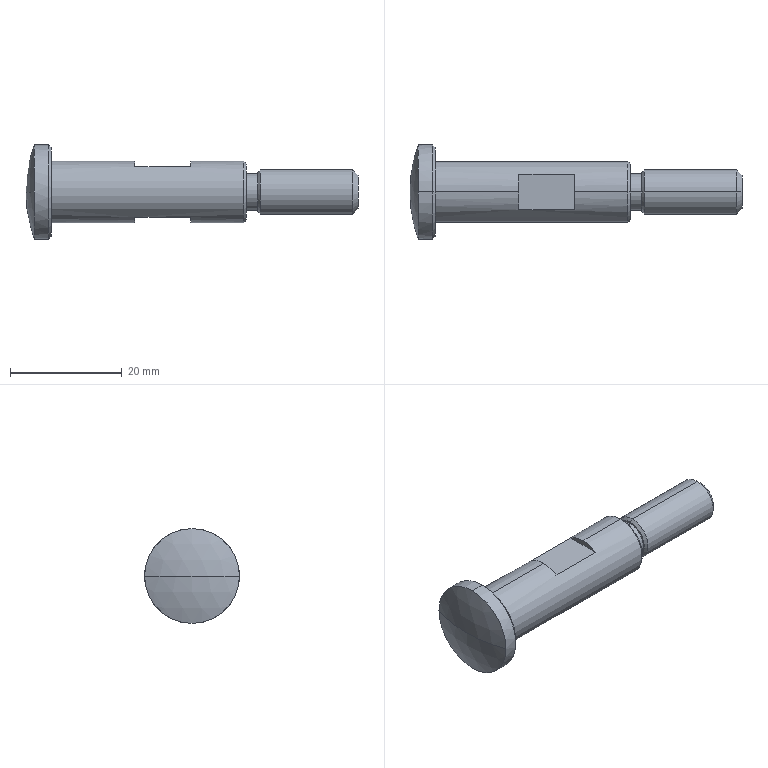Part | SolidWorks | features Chamfer 2, ICE 1, MirrorPattern 1, RefAxis 1, RevCut 1, Revolution 1 | 1 solid | 28 faces | box 59.5 x 17 x 17 mm | volume 5040 mm3 | plane 10 | cone 8 | cylinder 8 | sphere 2 | commonest cylinder face diameters 6.5 x2 8 x2 11 x2 17 x2
STEP:
#1=CARTESIAN_POINT('',(41.5,0.,3.5));
#2=VERTEX_POINT('',#1);
#3=CARTESIAN_POINT('',(41.5,0.,-3.5));
#4=VERTEX_POINT('',#3);
#5=CARTESIAN_POINT('',(41.5,0.,0.));
#6=DIRECTION('',(-1.,0.,0.));
#7=DIRECTION('',(0.,0.,-1.));
#8=AXIS2_PLACEMENT_3D('',#5,#6,#7);
#9=CIRCLE('',#8,3.5);
#10=EDGE_CURVE('',#2,#4,#9,.T.);
#11=ORIENTED_EDGE('',*,*,#10,.F.);
#12=CARTESIAN_POINT('',(42.,0.,4.));
#13=VERTEX_POINT('',#12);
#14=CARTESIAN_POINT('',(42.,0.,4.));
#15=DIRECTION('',(0.7071,0.,0.7071));
#16=VECTOR('',#15,1000.);
#17=LINE('',#14,#16);
#18=EDGE_CURVE('',#2,#13,#17,.T.);
#19=ORIENTED_EDGE('',*,*,#18,.T.);
#20=CARTESIAN_POINT('',(42.,0.,-4.));
#21=VERTEX_POINT('',#20);
#22=CARTESIAN_POINT('',(42.,0.,0.));
#23=DIRECTION('',(1.,0.,0.));
#24=DIRECTION('',(0.,0.,-1.));
#25=AXIS2_PLACEMENT_3D('',#22,#23,#24);
#26=CIRCLE('',#25,4.);
#27=EDGE_CURVE('',#21,#13,#26,.T.);
#28=ORIENTED_EDGE('',*,*,#27,.F.);
#29=CARTESIAN_POINT('',(42.,0.,-4.));
#30=DIRECTION('',(0.7071,0.,-0.7071));
#31=VECTOR('',#30,1000.);
#32=LINE('',#29,#31);
#33=EDGE_CURVE('',#4,#21,#32,.T.);
#34=ORIENTED_EDGE('',*,*,#33,.F.);
#35=EDGE_LOOP('',(#11,#19,#28,#34));
#36=FACE_OUTER_BOUND('',#35,.T.);
#37=CARTESIAN_POINT('',(42.,0.,0.));
#38=DIRECTION('',(1.,0.,0.));
#39=DIRECTION('',(0.,0.,-1.));
#40=AXIS2_PLACEMENT_3D('',#37,#38,#39);
#41=CONICAL_SURFACE('',#40,4.,0.7854);
#42=ADVANCED_FACE('',(#36),#41,.T.);
#43=CARTESIAN_POINT('',(58.5,0.,4.));
#44=VERTEX_POINT('',#43);
#45=CARTESIAN_POINT('',(58.5,0.,-4.));
#46=VERTEX_POINT('',#45);
#47=CARTESIAN_POINT('',(58.5,0.,0.));
#48=DIRECTION('',(-1.,0.,0.));
#49=DIRECTION('',(0.,0.,1.));
#50=AXIS2_PLACEMENT_3D('',#47,#48,#49);
#51=CIRCLE('',#50,4.);
#52=EDGE_CURVE('',#44,#46,#51,.T.);
#53=ORIENTED_EDGE('',*,*,#52,.T.);
#54=CARTESIAN_POINT('',(0.,0.,-4.));
#55=DIRECTION('',(-1.,0.,0.));
#56=VECTOR('',#55,1000.);
#57=LINE('',#54,#56);
#58=EDGE_CURVE('',#46,#21,#57,.T.);
#59=ORIENTED_EDGE('',*,*,#58,.T.);
#60=ORIENTED_EDGE('',*,*,#27,.T.);
#61=CARTESIAN_POINT('',(0.,0.,4.));
#62=DIRECTION('',(-1.,0.,0.));
#63=VECTOR('',#62,1000.);
#64=LINE('',#61,#63);
#65=EDGE_CURVE('',#44,#13,#64,.T.);
#66=ORIENTED_EDGE('',*,*,#65,.F.);
#67=EDGE_LOOP('',(#53,#59,#60,#66));
#68=FACE_OUTER_BOUND('',#67,.T.);
#69=CARTESIAN_POINT('',(0.,0.,0.));
#70=DIRECTION('',(-1.,0.,0.));
#71=DIRECTION('',(0.,0.,1.));
#72=AXIS2_PLACEMENT_3D('',#69,#70,#71);
#73=CYLINDRICAL_SURFACE('',#72,4.);
#74=ADVANCED_FACE('',(#68),#73,.T.);
#75=CARTESIAN_POINT('',(59.5,0.,3.));
#76=VERTEX_POINT('',#75);
#77=CARTESIAN_POINT('',(59.5,0.,-3.));
#78=VERTEX_POINT('',#77);
#79=CARTESIAN_POINT('',(59.5,0.,0.));
#80=DIRECTION('',(-1.,0.,0.));
#81=DIRECTION('',(0.,0.,1.));
#82=AXIS2_PLACEMENT_3D('',#79,#80,#81);
#83=CIRCLE('',#82,3.);
#84=EDGE_CURVE('',#76,#78,#83,.T.);
#85=ORIENTED_EDGE('',*,*,#84,.T.);
#86=CARTESIAN_POINT('',(59.5,0.,-3.));
#87=DIRECTION('',(-0.7071,0.,-0.7071));
#88=VECTOR('',#87,1000.);
#89=LINE('',#86,#88);
#90=EDGE_CURVE('',#78,#46,#89,.T.);
#91=ORIENTED_EDGE('',*,*,#90,.T.);
#92=ORIENTED_EDGE('',*,*,#52,.F.);
#93=CARTESIAN_POINT('',(59.5,0.,3.));
#94=DIRECTION('',(-0.7071,0.,0.7071));
#95=VECTOR('',#94,1000.);
#96=LINE('',#93,#95);
#97=EDGE_CURVE('',#76,#44,#96,.T.);
#98=ORIENTED_EDGE('',*,*,#97,.F.);
#99=EDGE_LOOP('',(#85,#91,#92,#98));
#100=FACE_OUTER_BOUND('',#99,.T.);
#101=CARTESIAN_POINT('',(59.5,0.,0.));
#102=DIRECTION('',(-1.,0.,0.));
#103=DIRECTION('',(0.,0.,1.));
#104=AXIS2_PLACEMENT_3D('',#101,#102,#103);
#105=CONICAL_SURFACE('',#104,3.,0.7854);
#106=ADVANCED_FACE('',(#100),#105,.T.);
#107=CARTESIAN_POINT('',(39.5,0.,-3.25));
#108=VERTEX_POINT('',#107);
#109=CARTESIAN_POINT('',(39.5,0.,3.25));
#110=VERTEX_POINT('',#109);
#111=CARTESIAN_POINT('',(39.5,0.,0.));
#112=DIRECTION('',(1.,0.,0.));
#113=DIRECTION('',(0.,0.,-1.));
#114=AXIS2_PLACEMENT_3D('',#111,#112,#113);
#115=CIRCLE('',#114,3.25);
#116=EDGE_CURVE('',#108,#110,#115,.T.);
#117=ORIENTED_EDGE('',*,*,#116,.T.);
#118=CARTESIAN_POINT('',(41.5,0.,3.25));
#119=VERTEX_POINT('',#118);
#120=CARTESIAN_POINT('',(58.5,0.,3.25));
#121=DIRECTION('',(1.,0.,0.));
#122=VECTOR('',#121,1000.);
#123=LINE('',#120,#122);
#124=EDGE_CURVE('',#110,#119,#123,.T.);
#125=ORIENTED_EDGE('',*,*,#124,.T.);
#126=CARTESIAN_POINT('',(41.5,0.,-3.25));
#127=VERTEX_POINT('',#126);
#128=CARTESIAN_POINT('',(41.5,0.,0.));
#129=DIRECTION('',(1.,0.,0.));
#130=DIRECTION('',(0.,0.,-1.));
#131=AXIS2_PLACEMENT_3D('',#128,#129,#130);
#132=CIRCLE('',#131,3.25);
#133=EDGE_CURVE('',#127,#119,#132,.T.);
#134=ORIENTED_EDGE('',*,*,#133,.F.);
#135=CARTESIAN_POINT('',(58.5,0.,-3.25));
#136=DIRECTION('',(1.,0.,0.));
#137=VECTOR('',#136,1000.);
#138=LINE('',#135,#137);
#139=EDGE_CURVE('',#108,#127,#138,.T.);
#140=ORIENTED_EDGE('',*,*,#139,.F.);
#141=EDGE_LOOP('',(#117,#125,#134,#140));
#142=FACE_OUTER_BOUND('',#141,.T.);
#143=CARTESIAN_POINT('',(58.5,0.,0.));
#144=DIRECTION('',(1.,0.,0.));
#145=DIRECTION('',(0.,0.,-1.));
#146=AXIS2_PLACEMENT_3D('',#143,#144,#145);
#147=CYLINDRICAL_SURFACE('',#146,3.25);
#148=ADVANCED_FACE('',(#142),#147,.T.);
#149=CARTESIAN_POINT('',(4.5,0.,-8.));
#150=VERTEX_POINT('',#149);
#151=CARTESIAN_POINT('',(4.5,0.,8.));
#152=VERTEX_POINT('',#151);
#153=CARTESIAN_POINT('',(4.5,0.,0.));
#154=DIRECTION('',(1.,0.,0.));
#155=DIRECTION('',(0.,0.,1.));
#156=AXIS2_PLACEMENT_3D('',#153,#154,#155);
#157=CIRCLE('',#156,8.);
#158=EDGE_CURVE('',#150,#152,#157,.T.);
#159=ORIENTED_EDGE('',*,*,#158,.F.);
#160=CARTESIAN_POINT('',(4.,0.,-8.5));
#161=VERTEX_POINT('',#160);
#162=CARTESIAN_POINT('',(4.,0.,-8.5));
#163=DIRECTION('',(-0.7071,0.,-0.7071));
#164=VECTOR('',#163,1000.);
#165=LINE('',#162,#164);
#166=EDGE_CURVE('',#150,#161,#165,.T.);
#167=ORIENTED_EDGE('',*,*,#166,.T.);
#168=CARTESIAN_POINT('',(4.,0.,8.5));
#169=VERTEX_POINT('',#168);
#170=CARTESIAN_POINT('',(4.,0.,0.));
#171=DIRECTION('',(-1.,0.,0.));
#172=DIRECTION('',(0.,0.,1.));
#173=AXIS2_PLACEMENT_3D('',#170,#171,#172);
#174=CIRCLE('',#173,8.5);
#175=EDGE_CURVE('',#169,#161,#174,.T.);
#176=ORIENTED_EDGE('',*,*,#175,.F.);
#177=CARTESIAN_POINT('',(4.,0.,8.5));
#178=DIRECTION('',(-0.7071,0.,0.7071));
#179=VECTOR('',#178,1000.);
#180=LINE('',#177,#179);
#181=EDGE_CURVE('',#152,#169,#180,.T.);
#182=ORIENTED_EDGE('',*,*,#181,.F.);
#183=EDGE_LOOP('',(#159,#167,#176,#182));
#184=FACE_OUTER_BOUND('',#183,.T.);
#185=CARTESIAN_POINT('',(4.,0.,0.));
#186=DIRECTION('',(-1.,0.,0.));
#187=DIRECTION('',(0.,0.,1.));
#188=AXIS2_PLACEMENT_3D('',#185,#186,#187);
#189=CONICAL_SURFACE('',#188,8.5,0.7854);
#190=ADVANCED_FACE('',(#184),#189,.T.);
#191=CARTESIAN_POINT('',(39.5,0.,-5.));
#192=VERTEX_POINT('',#191);
#193=CARTESIAN_POINT('',(39.5,0.,5.));
#194=VERTEX_POINT('',#193);
#195=CARTESIAN_POINT('',(39.5,0.,0.));
#196=DIRECTION('',(1.,0.,0.));
#197=DIRECTION('',(0.,0.,1.));
#198=AXIS2_PLACEMENT_3D('',#195,#196,#197);
#199=CIRCLE('',#198,5.);
#200=EDGE_CURVE('',#192,#194,#199,.T.);
#201=ORIENTED_EDGE('',*,*,#200,.F.);
#202=CARTESIAN_POINT('',(39.,0.,-5.5));
#203=VERTEX_POINT('',#202);
#204=CARTESIAN_POINT('',(39.,0.,-5.5));
#205=DIRECTION('',(-0.7071,0.,-0.7071));
#206=VECTOR('',#205,1000.);
#207=LINE('',#204,#206);
#208=EDGE_CURVE('',#192,#203,#207,.T.);
#209=ORIENTED_EDGE('',*,*,#208,.T.);
#210=CARTESIAN_POINT('',(39.,0.,5.5));
#211=VERTEX_POINT('',#210);
#212=CARTESIAN_POINT('',(39.,0.,0.));
#213=DIRECTION('',(-1.,0.,0.));
#214=DIRECTION('',(0.,0.,1.));
#215=AXIS2_PLACEMENT_3D('',#212,#213,#214);
#216=CIRCLE('',#215,5.5);
#217=EDGE_CURVE('',#211,#203,#216,.T.);
#218=ORIENTED_EDGE('',*,*,#217,.F.);
#219=CARTESIAN_POINT('',(39.,0.,5.5));
#220=DIRECTION('',(-0.7071,0.,0.7071));
#221=VECTOR('',#220,1000.);
#222=LINE('',#219,#221);
#223=EDGE_CURVE('',#194,#211,#222,.T.);
#224=ORIENTED_EDGE('',*,*,#223,.F.);
#225=EDGE_LOOP('',(#201,#209,#218,#224));
#226=FACE_OUTER_BOUND('',#225,.T.);
#227=CARTESIAN_POINT('',(39.,0.,0.));
#228=DIRECTION('',(-1.,0.,0.));
#229=DIRECTION('',(0.,0.,1.));
#230=AXIS2_PLACEMENT_3D('',#227,#228,#229);
#231=CONICAL_SURFACE('',#230,5.5,0.7854);
#232=ADVANCED_FACE('',(#226),#231,.T.);
#233=ORIENTED_EDGE('',*,*,#175,.T.);
#234=CARTESIAN_POINT('',(1.489,0.,-8.5));
#235=VERTEX_POINT('',#234);
#236=CARTESIAN_POINT('',(0.,0.,-8.5));
#237=DIRECTION('',(-1.,0.,0.));
#238=VECTOR('',#237,1000.);
#239=LINE('',#236,#238);
#240=EDGE_CURVE('',#161,#235,#239,.T.);
#241=ORIENTED_EDGE('',*,*,#240,.T.);
#242=CARTESIAN_POINT('',(1.489,8.5,0.));
#243=VERTEX_POINT('',#242);
#244=CARTESIAN_POINT('',(1.489,0.,0.));
#245=DIRECTION('',(-1.,0.,0.));
#246=DIRECTION('',(0.,0.,1.));
#247=AXIS2_PLACEMENT_3D('',#244,#245,#246);
#248=CIRCLE('',#247,8.5);
#249=EDGE_CURVE('',#243,#235,#248,.T.);
#250=ORIENTED_EDGE('',*,*,#249,.F.);
#251=CARTESIAN_POINT('',(1.489,0.,8.5));
#252=VERTEX_POINT('',#251);
#253=CARTESIAN_POINT('',(1.489,0.,0.));
#254=DIRECTION('',(-1.,0.,0.));
#255=DIRECTION('',(0.,0.,1.));
#256=AXIS2_PLACEMENT_3D('',#253,#254,#255);
#257=CIRCLE('',#256,8.5);
#258=EDGE_CURVE('',#252,#243,#257,.T.);
#259=ORIENTED_EDGE('',*,*,#258,.F.);
#260=CARTESIAN_POINT('',(0.,0.,8.5));
#261=DIRECTION('',(-1.,0.,0.));
#262=VECTOR('',#261,1000.);
#263=LINE('',#260,#262);
#264=EDGE_CURVE('',#169,#252,#263,.T.);
#265=ORIENTED_EDGE('',*,*,#264,.F.);
#266=EDGE_LOOP('',(#233,#241,#250,#259,#265));
#267=FACE_OUTER_BOUND('',#266,.T.);
#268=CARTESIAN_POINT('',(0.,0.,0.));
#269=DIRECTION('',(-1.,0.,0.));
#270=DIRECTION('',(0.,0.,1.));
#271=AXIS2_PLACEMENT_3D('',#268,#269,#270);
#272=CYLINDRICAL_SURFACE('',#271,8.5);
#273=ADVANCED_FACE('',(#267),#272,.T.);
#274=ORIENTED_EDGE('',*,*,#249,.T.);
#275=CARTESIAN_POINT('',(1.489,-8.5,0.));
#276=VERTEX_POINT('',#275);
#277=CARTESIAN_POINT('',(1.489,0.,0.));
#278=DIRECTION('',(-1.,0.,0.));
#279=DIRECTION('',(0.,0.,1.));
#280=AXIS2_PLACEMENT_3D('',#277,#278,#279);
#281=CIRCLE('',#280,8.5);
#282=EDGE_CURVE('',#235,#276,#281,.T.);
#283=ORIENTED_EDGE('',*,*,#282,.T.);
#284=CARTESIAN_POINT('',(0.,0.,0.));
#285=VERTEX_POINT('',#284);
#286=CARTESIAN_POINT('',(25.,0.,0.));
#287=DIRECTION('',(0.,0.,-1.));
#288=DIRECTION('',(0.,1.,0.));
#289=AXIS2_PLACEMENT_3D('',#286,#287,#288);
#290=CIRCLE('',#289,25.);
#291=EDGE_CURVE('',#276,#285,#290,.T.);
#292=ORIENTED_EDGE('',*,*,#291,.T.);
#293=CARTESIAN_POINT('',(25.,0.,0.));
#294=DIRECTION('',(0.,0.,1.));
#295=DIRECTION('',(1.,0.,0.));
#296=AXIS2_PLACEMENT_3D('',#293,#294,#295);
#297=CIRCLE('',#296,25.);
#298=EDGE_CURVE('',#243,#285,#297,.T.);
#299=ORIENTED_EDGE('',*,*,#298,.F.);
#300=EDGE_LOOP('',(#274,#283,#292,#299));
#301=FACE_OUTER_BOUND('',#300,.T.);
#302=CARTESIAN_POINT('',(25.,0.,0.));
#303=DIRECTION('',(0.,0.,-1.));
#304=DIRECTION('',(0.,1.,0.));
#305=AXIS2_PLACEMENT_3D('',#302,#303,#304);
#306=SPHERICAL_SURFACE('',#305,25.);
#307=ADVANCED_FACE('',(#301),#306,.T.);
#308=ORIENTED_EDGE('',*,*,#217,.T.);
#309=CARTESIAN_POINT('',(29.5,0.,-5.5));
#310=VERTEX_POINT('',#309);
#311=CARTESIAN_POINT('',(0.,0.,-5.5));
#312=DIRECTION('',(-1.,0.,0.));
#313=VECTOR('',#312,1000.);
#314=LINE('',#311,#313);
#315=EDGE_CURVE('',#203,#310,#314,.T.);
#316=ORIENTED_EDGE('',*,*,#315,.T.);
#317=CARTESIAN_POINT('',(29.5,3.162,-4.5));
#318=VERTEX_POINT('',#317);
#319=CARTESIAN_POINT('',(29.5,0.,0.));
#320=DIRECTION('',(1.,0.,0.));
#321=DIRECTION('',(0.,0.,-1.));
#322=AXIS2_PLACEMENT_3D('',#319,#320,#321);
#323=CIRCLE('',#322,5.5);
#324=EDGE_CURVE('',#310,#318,#323,.T.);
#325=ORIENTED_EDGE('',*,*,#324,.T.);
#326=CARTESIAN_POINT('',(19.5,3.162,-4.5));
#327=VERTEX_POINT('',#326);
#328=CARTESIAN_POINT('',(0.,3.162,-4.5));
#329=DIRECTION('',(-1.,0.,0.));
#330=VECTOR('',#329,1000.);
#331=LINE('',#328,#330);
#332=EDGE_CURVE('',#318,#327,#331,.T.);
#333=ORIENTED_EDGE('',*,*,#332,.T.);
#334=CARTESIAN_POINT('',(19.5,0.,-5.5));
#335=VERTEX_POINT('',#334);
#336=CARTESIAN_POINT('',(19.5,0.,0.));
#337=DIRECTION('',(-1.,0.,0.));
#338=DIRECTION('',(0.,0.,1.));
#339=AXIS2_PLACEMENT_3D('',#336,#337,#338);
#340=CIRCLE('',#339,5.5);
#341=EDGE_CURVE('',#327,#335,#340,.T.);
#342=ORIENTED_EDGE('',*,*,#341,.T.);
#343=CARTESIAN_POINT('',(4.5,0.,-5.5));
#344=VERTEX_POINT('',#343);
#345=CARTESIAN_POINT('',(0.,0.,-5.5));
#346=DIRECTION('',(-1.,0.,0.));
#347=VECTOR('',#346,1000.);
#348=LINE('',#345,#347);
#349=EDGE_CURVE('',#335,#344,#348,.T.);
#350=ORIENTED_EDGE('',*,*,#349,.T.);
#351=CARTESIAN_POINT('',(4.5,0.,5.5));
#352=VERTEX_POINT('',#351);
#353=CARTESIAN_POINT('',(4.5,0.,0.));
#354=DIRECTION('',(-1.,0.,0.));
#355=DIRECTION('',(0.,0.,1.));
#356=AXIS2_PLACEMENT_3D('',#353,#354,#355);
#357=CIRCLE('',#356,5.5);
#358=EDGE_CURVE('',#352,#344,#357,.T.);
#359=ORIENTED_EDGE('',*,*,#358,.F.);
#360=CARTESIAN_POINT('',(19.5,0.,5.5));
#361=VERTEX_POINT('',#360);
#362=CARTESIAN_POINT('',(0.,0.,5.5));
#363=DIRECTION('',(-1.,0.,0.));
#364=VECTOR('',#363,1000.);
#365=LINE('',#362,#364);
#366=EDGE_CURVE('',#361,#352,#365,.T.);
#367=ORIENTED_EDGE('',*,*,#366,.F.);
#368=CARTESIAN_POINT('',(19.5,3.162,4.5));
#369=VERTEX_POINT('',#368);
#370=CARTESIAN_POINT('',(19.5,0.,0.));
#371=DIRECTION('',(1.,0.,0.));
#372=DIRECTION('',(0.,0.,-1.));
#373=AXIS2_PLACEMENT_3D('',#370,#371,#372);
#374=CIRCLE('',#373,5.5);
#375=EDGE_CURVE('',#369,#361,#374,.T.);
#376=ORIENTED_EDGE('',*,*,#375,.F.);
#377=CARTESIAN_POINT('',(29.5,3.162,4.5));
#378=VERTEX_POINT('',#377);
#379=CARTESIAN_POINT('',(0.,3.162,4.5));
#380=DIRECTION('',(-1.,0.,0.));
#381=VECTOR('',#380,1000.);
#382=LINE('',#379,#381);
#383=EDGE_CURVE('',#378,#369,#382,.T.);
#384=ORIENTED_EDGE('',*,*,#383,.F.);
#385=CARTESIAN_POINT('',(29.5,0.,5.5));
#386=VERTEX_POINT('',#385);
#387=CARTESIAN_POINT('',(29.5,0.,0.));
#388=DIRECTION('',(-1.,0.,0.));
#389=DIRECTION('',(0.,0.,1.));
#390=AXIS2_PLACEMENT_3D('',#387,#388,#389);
#391=CIRCLE('',#390,5.5);
#392=EDGE_CURVE('',#386,#378,#391,.T.);
#393=ORIENTED_EDGE('',*,*,#392,.F.);
#394=CARTESIAN_POINT('',(0.,0.,5.5));
#395=DIRECTION('',(-1.,0.,0.));
#396=VECTOR('',#395,1000.);
#397=LINE('',#394,#396);
#398=EDGE_CURVE('',#211,#386,#397,.T.);
#399=ORIENTED_EDGE('',*,*,#398,.F.);
#400=EDGE_LOOP('',(#308,#316,#325,#333,#342,#350,#359,#367,#376,#384,#393,#399));
#401=FACE_OUTER_BOUND('',#400,.T.);
#402=CARTESIAN_POINT('',(0.,0.,0.));
#403=DIRECTION('',(-1.,0.,0.));
#404=DIRECTION('',(0.,0.,1.));
#405=AXIS2_PLACEMENT_3D('',#402,#403,#404);
#406=CYLINDRICAL_SURFACE('',#405,5.5);
#407=ADVANCED_FACE('',(#401),#406,.T.);
#408=ORIENTED_EDGE('',*,*,#315,.F.);
#409=CARTESIAN_POINT('',(39.,0.,0.));
#410=DIRECTION('',(-1.,0.,0.));
#411=DIRECTION('',(0.,0.,1.));
#412=AXIS2_PLACEMENT_3D('',#409,#410,#411);
#413=CIRCLE('',#412,5.5);
#414=EDGE_CURVE('',#203,#211,#413,.T.);
#415=ORIENTED_EDGE('',*,*,#414,.T.);
#416=ORIENTED_EDGE('',*,*,#398,.T.);
#417=CARTESIAN_POINT('',(29.5,-3.162,4.5));
#418=VERTEX_POINT('',#417);
#419=CARTESIAN_POINT('',(29.5,0.,0.));
#420=DIRECTION('',(-1.,0.,0.));
#421=DIRECTION('',(0.,0.,1.));
#422=AXIS2_PLACEMENT_3D('',#419,#420,#421);
#423=CIRCLE('',#422,5.5);
#424=EDGE_CURVE('',#418,#386,#423,.T.);
#425=ORIENTED_EDGE('',*,*,#424,.F.);
#426=CARTESIAN_POINT('',(19.5,-3.162,4.5));
#427=VERTEX_POINT('',#426);
#428=CARTESIAN_POINT('',(0.,-3.162,4.5));
#429=DIRECTION('',(1.,0.,0.));
#430=VECTOR('',#429,1000.);
#431=LINE('',#428,#430);
#432=EDGE_CURVE('',#427,#418,#431,.T.);
#433=ORIENTED_EDGE('',*,*,#432,.F.);
#434=CARTESIAN_POINT('',(19.5,0.,0.));
#435=DIRECTION('',(1.,0.,0.));
#436=DIRECTION('',(0.,0.,-1.));
#437=AXIS2_PLACEMENT_3D('',#434,#435,#436);
#438=CIRCLE('',#437,5.5);
#439=EDGE_CURVE('',#361,#427,#438,.T.);
#440=ORIENTED_EDGE('',*,*,#439,.F.);
#441=ORIENTED_EDGE('',*,*,#366,.T.);
#442=CARTESIAN_POINT('',(4.5,0.,0.));
#443=DIRECTION('',(-1.,0.,0.));
#444=DIRECTION('',(0.,0.,1.));
#445=AXIS2_PLACEMENT_3D('',#442,#443,#444);
#446=CIRCLE('',#445,5.5);
#447=EDGE_CURVE('',#344,#352,#446,.T.);
#448=ORIENTED_EDGE('',*,*,#447,.F.);
#449=ORIENTED_EDGE('',*,*,#349,.F.);
#450=CARTESIAN_POINT('',(19.5,-3.162,-4.5));
#451=VERTEX_POINT('',#450);
#452=CARTESIAN_POINT('',(19.5,0.,0.));
#453=DIRECTION('',(-1.,0.,0.));
#454=DIRECTION('',(0.,0.,1.));
#455=AXIS2_PLACEMENT_3D('',#452,#453,#454);
#456=CIRCLE('',#455,5.5);
#457=EDGE_CURVE('',#335,#451,#456,.T.);
#458=ORIENTED_EDGE('',*,*,#457,.T.);
#459=CARTESIAN_POINT('',(29.5,-3.162,-4.5));
#460=VERTEX_POINT('',#459);
#461=CARTESIAN_POINT('',(0.,-3.162,-4.5));
#462=DIRECTION('',(1.,0.,0.));
#463=VECTOR('',#462,1000.);
#464=LINE('',#461,#463);
#465=EDGE_CURVE('',#451,#460,#464,.T.);
#466=ORIENTED_EDGE('',*,*,#465,.T.);
#467=CARTESIAN_POINT('',(29.5,0.,0.));
#468=DIRECTION('',(1.,0.,0.));
#469=DIRECTION('',(0.,0.,-1.));
#470=AXIS2_PLACEMENT_3D('',#467,#468,#469);
#471=CIRCLE('',#470,5.5);
#472=EDGE_CURVE('',#460,#310,#471,.T.);
#473=ORIENTED_EDGE('',*,*,#472,.T.);
#474=EDGE_LOOP('',(#408,#415,#416,#425,#433,#440,#441,#448,#449,#458,#466,#473));
#475=FACE_OUTER_BOUND('',#474,.T.);
#476=CARTESIAN_POINT('',(0.,0.,0.));
#477=DIRECTION('',(-1.,0.,0.));
#478=DIRECTION('',(0.,0.,1.));
#479=AXIS2_PLACEMENT_3D('',#476,#477,#478);
#480=CYLINDRICAL_SURFACE('',#479,5.5);
#481=ADVANCED_FACE('',(#475),#480,.T.);
#482=ORIENTED_EDGE('',*,*,#291,.F.);
#483=CARTESIAN_POINT('',(1.489,0.,0.));
#484=DIRECTION('',(-1.,0.,0.));
#485=DIRECTION('',(0.,0.,1.));
#486=AXIS2_PLACEMENT_3D('',#483,#484,#485);
#487=CIRCLE('',#486,8.5);
#488=EDGE_CURVE('',#276,#252,#487,.T.);
#489=ORIENTED_EDGE('',*,*,#488,.T.);
#490=ORIENTED_EDGE('',*,*,#258,.T.);
#491=ORIENTED_EDGE('',*,*,#298,.T.);
#492=EDGE_LOOP('',(#482,#489,#490,#491));
#493=FACE_OUTER_BOUND('',#492,.T.);
#494=CARTESIAN_POINT('',(25.,0.,0.));
#495=DIRECTION('',(0.,0.,-1.));
#496=DIRECTION('',(0.,1.,0.));
#497=AXIS2_PLACEMENT_3D('',#494,#495,#496);
#498=SPHERICAL_SURFACE('',#497,25.);
#499=ADVANCED_FACE('',(#493),#498,.T.);
#500=CARTESIAN_POINT('',(39.5,0.,0.));
#501=DIRECTION('',(1.,0.,0.));
#502=DIRECTION('',(0.,0.,1.));
#503=AXIS2_PLACEMENT_3D('',#500,#501,#502);
#504=CIRCLE('',#503,5.);
#505=EDGE_CURVE('',#194,#192,#504,.T.);
#506=ORIENTED_EDGE('',*,*,#505,.T.);
#507=ORIENTED_EDGE('',*,*,#200,.T.);
#508=EDGE_LOOP('',(#506,#507));
#509=FACE_OUTER_BOUND('',#508,.T.);
#510=ORIENTED_EDGE('',*,*,#116,.F.);
#511=CARTESIAN_POINT('',(39.5,0.,0.));
#512=DIRECTION('',(1.,0.,0.));
#513=DIRECTION('',(0.,0.,-1.));
#514=AXIS2_PLACEMENT_3D('',#511,#512,#513);
#515=CIRCLE('',#514,3.25);
#516=EDGE_CURVE('',#110,#108,#515,.T.);
#517=ORIENTED_EDGE('',*,*,#516,.F.);
#518=EDGE_LOOP('',(#510,#517));
#519=FACE_BOUND('',#518,.T.);
#520=CARTESIAN_POINT('',(39.5,4.,0.));
#521=DIRECTION('',(-1.,0.,0.));
#522=DIRECTION('',(0.,0.,1.));
#523=AXIS2_PLACEMENT_3D('',#520,#521,#522);
#524=PLANE('',#523);
#525=ADVANCED_FACE('',(#509,#519),#524,.F.);
#526=CARTESIAN_POINT('',(4.5,0.,0.));
#527=DIRECTION('',(1.,0.,0.));
#528=DIRECTION('',(0.,0.,1.));
#529=AXIS2_PLACEMENT_3D('',#526,#527,#528);
#530=CIRCLE('',#529,8.);
#531=EDGE_CURVE('',#152,#150,#530,.T.);
#532=ORIENTED_EDGE('',*,*,#531,.T.);
#533=ORIENTED_EDGE('',*,*,#158,.T.);
#534=EDGE_LOOP('',(#532,#533));
#535=FACE_OUTER_BOUND('',#534,.T.);
#536=ORIENTED_EDGE('',*,*,#358,.T.);
#537=ORIENTED_EDGE('',*,*,#447,.T.);
#538=EDGE_LOOP('',(#536,#537));
#539=FACE_BOUND('',#538,.T.);
#540=CARTESIAN_POINT('',(4.5,5.5,0.));
#541=DIRECTION('',(-1.,0.,0.));
#542=DIRECTION('',(0.,0.,1.));
#543=AXIS2_PLACEMENT_3D('',#540,#541,#542);
#544=PLANE('',#543);
#545=ADVANCED_FACE('',(#535,#539),#544,.F.);
#546=ORIENTED_EDGE('',*,*,#240,.F.);
#547=CARTESIAN_POINT('',(4.,0.,0.));
#548=DIRECTION('',(-1.,0.,0.));
#549=DIRECTION('',(0.,0.,1.));
#550=AXIS2_PLACEMENT_3D('',#547,#548,#549);
#551=CIRCLE('',#550,8.5);
#552=EDGE_CURVE('',#161,#169,#551,.T.);
#553=ORIENTED_EDGE('',*,*,#552,.T.);
#554=ORIENTED_EDGE('',*,*,#264,.T.);
#555=ORIENTED_EDGE('',*,*,#488,.F.);
#556=ORIENTED_EDGE('',*,*,#282,.F.);
#557=EDGE_LOOP('',(#546,#553,#554,#555,#556));
#558=FACE_OUTER_BOUND('',#557,.T.);
#559=CARTESIAN_POINT('',(0.,0.,0.));
#560=DIRECTION('',(-1.,0.,0.));
#561=DIRECTION('',(0.,0.,1.));
#562=AXIS2_PLACEMENT_3D('',#559,#560,#561);
#563=CYLINDRICAL_SURFACE('',#562,8.5);
#564=ADVANCED_FACE('',(#558),#563,.T.);
#565=CARTESIAN_POINT('',(19.5,-5.,-4.5));
#566=DIRECTION('',(0.,1.,0.));
#567=VECTOR('',#566,1000.);
#568=LINE('',#565,#567);
#569=EDGE_CURVE('',#451,#327,#568,.T.);
#570=ORIENTED_EDGE('',*,*,#569,.F.);
#571=ORIENTED_EDGE('',*,*,#457,.F.);
#572=ORIENTED_EDGE('',*,*,#341,.F.);
#573=EDGE_LOOP('',(#570,#571,#572));
#574=FACE_OUTER_BOUND('',#573,.T.);
#575=CARTESIAN_POINT('',(19.5,-5.,-5.5));
#576=DIRECTION('',(-1.,0.,0.));
#577=DIRECTION('',(0.,0.,1.));
#578=AXIS2_PLACEMENT_3D('',#575,#576,#577);
#579=PLANE('',#578);
#580=ADVANCED_FACE('',(#574),#579,.F.);
#581=ORIENTED_EDGE('',*,*,#472,.F.);
#582=CARTESIAN_POINT('',(29.5,-5.,-4.5));
#583=DIRECTION('',(0.,1.,0.));
#584=VECTOR('',#583,1000.);
#585=LINE('',#582,#584);
#586=EDGE_CURVE('',#460,#318,#585,.T.);
#587=ORIENTED_EDGE('',*,*,#586,.T.);
#588=ORIENTED_EDGE('',*,*,#324,.F.);
#589=EDGE_LOOP('',(#581,#587,#588));
#590=FACE_OUTER_BOUND('',#589,.T.);
#591=CARTESIAN_POINT('',(29.5,-5.,-5.5));
#592=DIRECTION('',(1.,0.,0.));
#593=DIRECTION('',(0.,0.,-1.));
#594=AXIS2_PLACEMENT_3D('',#591,#592,#593);
#595=PLANE('',#594);
#596=ADVANCED_FACE('',(#590),#595,.F.);
#597=ORIENTED_EDGE('',*,*,#586,.F.);
#598=ORIENTED_EDGE('',*,*,#465,.F.);
#599=ORIENTED_EDGE('',*,*,#569,.T.);
#600=ORIENTED_EDGE('',*,*,#332,.F.);
#601=EDGE_LOOP('',(#597,#598,#599,#600));
#602=FACE_OUTER_BOUND('',#601,.T.);
#603=CARTESIAN_POINT('',(19.5,-5.,-4.5));
#604=DIRECTION('',(0.,0.,1.));
#605=DIRECTION('',(1.,0.,0.));
#606=AXIS2_PLACEMENT_3D('',#603,#604,#605);
#607=PLANE('',#606);
#608=ADVANCED_FACE('',(#602),#607,.F.);
#609=CARTESIAN_POINT('',(19.5,-5.,4.5));
#610=DIRECTION('',(0.,1.,0.));
#611=VECTOR('',#610,1000.);
#612=LINE('',#609,#611);
#613=EDGE_CURVE('',#427,#369,#612,.T.);
#614=ORIENTED_EDGE('',*,*,#613,.T.);
#615=ORIENTED_EDGE('',*,*,#375,.T.);
#616=ORIENTED_EDGE('',*,*,#439,.T.);
#617=EDGE_LOOP('',(#614,#615,#616));
#618=FACE_OUTER_BOUND('',#617,.T.);
#619=CARTESIAN_POINT('',(19.5,-5.,5.5));
#620=DIRECTION('',(1.,0.,0.));
#621=DIRECTION('',(0.,0.,-1.));
#622=AXIS2_PLACEMENT_3D('',#619,#620,#621);
#623=PLANE('',#622);
#624=ADVANCED_FACE('',(#618),#623,.T.);
#625=ORIENTED_EDGE('',*,*,#383,.T.);
#626=ORIENTED_EDGE('',*,*,#613,.F.);
#627=ORIENTED_EDGE('',*,*,#432,.T.);
#628=CARTESIAN_POINT('',(29.5,-5.,4.5));
#629=DIRECTION('',(0.,1.,0.));
#630=VECTOR('',#629,1000.);
#631=LINE('',#628,#630);
#632=EDGE_CURVE('',#418,#378,#631,.T.);
#633=ORIENTED_EDGE('',*,*,#632,.T.);
#634=EDGE_LOOP('',(#625,#626,#627,#633));
#635=FACE_OUTER_BOUND('',#634,.T.);
#636=CARTESIAN_POINT('',(19.5,-5.,4.5));
#637=DIRECTION('',(0.,0.,1.));
#638=DIRECTION('',(1.,0.,0.));
#639=AXIS2_PLACEMENT_3D('',#636,#637,#638);
#640=PLANE('',#639);
#641=ADVANCED_FACE('',(#635),#640,.T.);
#642=ORIENTED_EDGE('',*,*,#424,.T.);
#643=ORIENTED_EDGE('',*,*,#392,.T.);
#644=ORIENTED_EDGE('',*,*,#632,.F.);
#645=EDGE_LOOP('',(#642,#643,#644));
#646=FACE_OUTER_BOUND('',#645,.T.);
#647=CARTESIAN_POINT('',(29.5,-5.,5.5));
#648=DIRECTION('',(-1.,0.,0.));
#649=DIRECTION('',(0.,0.,1.));
#650=AXIS2_PLACEMENT_3D('',#647,#648,#649);
#651=PLANE('',#650);
#652=ADVANCED_FACE('',(#646),#651,.T.);
#653=ORIENTED_EDGE('',*,*,#208,.F.);
#654=ORIENTED_EDGE('',*,*,#505,.F.);
#655=ORIENTED_EDGE('',*,*,#223,.T.);
#656=ORIENTED_EDGE('',*,*,#414,.F.);
#657=EDGE_LOOP('',(#653,#654,#655,#656));
#658=FACE_OUTER_BOUND('',#657,.T.);
#659=CARTESIAN_POINT('',(39.,0.,0.));
#660=DIRECTION('',(-1.,0.,0.));
#661=DIRECTION('',(0.,0.,1.));
#662=AXIS2_PLACEMENT_3D('',#659,#660,#661);
#663=CONICAL_SURFACE('',#662,5.5,0.7854);
#664=ADVANCED_FACE('',(#658),#663,.T.);
#665=ORIENTED_EDGE('',*,*,#166,.F.);
#666=ORIENTED_EDGE('',*,*,#531,.F.);
#667=ORIENTED_EDGE('',*,*,#181,.T.);
#668=ORIENTED_EDGE('',*,*,#552,.F.);
#669=EDGE_LOOP('',(#665,#666,#667,#668));
#670=FACE_OUTER_BOUND('',#669,.T.);
#671=CARTESIAN_POINT('',(4.,0.,0.));
#672=DIRECTION('',(-1.,0.,0.));
#673=DIRECTION('',(0.,0.,1.));
#674=AXIS2_PLACEMENT_3D('',#671,#672,#673);
#675=CONICAL_SURFACE('',#674,8.5,0.7854);
#676=ADVANCED_FACE('',(#670),#675,.T.);
#677=ORIENTED_EDGE('',*,*,#124,.F.);
#678=ORIENTED_EDGE('',*,*,#516,.T.);
#679=ORIENTED_EDGE('',*,*,#139,.T.);
#680=CARTESIAN_POINT('',(41.5,0.,0.));
#681=DIRECTION('',(1.,0.,0.));
#682=DIRECTION('',(0.,0.,-1.));
#683=AXIS2_PLACEMENT_3D('',#680,#681,#682);
#684=CIRCLE('',#683,3.25);
#685=EDGE_CURVE('',#119,#127,#684,.T.);
#686=ORIENTED_EDGE('',*,*,#685,.F.);
#687=EDGE_LOOP('',(#677,#678,#679,#686));
#688=FACE_OUTER_BOUND('',#687,.T.);
#689=CARTESIAN_POINT('',(58.5,0.,0.));
#690=DIRECTION('',(1.,0.,0.));
#691=DIRECTION('',(0.,0.,-1.));
#692=AXIS2_PLACEMENT_3D('',#689,#690,#691);
#693=CYLINDRICAL_SURFACE('',#692,3.25);
#694=ADVANCED_FACE('',(#688),#693,.T.);
#695=CARTESIAN_POINT('',(41.5,0.,0.));
#696=DIRECTION('',(-1.,0.,0.));
#697=DIRECTION('',(0.,0.,-1.));
#698=AXIS2_PLACEMENT_3D('',#695,#696,#697);
#699=CIRCLE('',#698,3.5);
#700=EDGE_CURVE('',#4,#2,#699,.T.);
#701=ORIENTED_EDGE('',*,*,#700,.T.);
#702=ORIENTED_EDGE('',*,*,#10,.T.);
#703=EDGE_LOOP('',(#701,#702));
#704=FACE_OUTER_BOUND('',#703,.T.);
#705=ORIENTED_EDGE('',*,*,#133,.T.);
#706=ORIENTED_EDGE('',*,*,#685,.T.);
#707=EDGE_LOOP('',(#705,#706));
#708=FACE_BOUND('',#707,.T.);
#709=CARTESIAN_POINT('',(41.5,0.,-4.));
#710=DIRECTION('',(1.,0.,0.));
#711=DIRECTION('',(0.,0.,-1.));
#712=AXIS2_PLACEMENT_3D('',#709,#710,#711);
#713=PLANE('',#712);
#714=ADVANCED_FACE('',(#704,#708),#713,.F.);
#715=ORIENTED_EDGE('',*,*,#84,.F.);
#716=CARTESIAN_POINT('',(59.5,0.,0.));
#717=DIRECTION('',(-1.,0.,0.));
#718=DIRECTION('',(0.,0.,1.));
#719=AXIS2_PLACEMENT_3D('',#716,#717,#718);
#720=CIRCLE('',#719,3.);
#721=EDGE_CURVE('',#78,#76,#720,.T.);
#722=ORIENTED_EDGE('',*,*,#721,.F.);
#723=EDGE_LOOP('',(#715,#722));
#724=FACE_OUTER_BOUND('',#723,.T.);
#725=CARTESIAN_POINT('',(59.5,0.,0.));
#726=DIRECTION('',(-1.,0.,0.));
#727=DIRECTION('',(0.,0.,1.));
#728=AXIS2_PLACEMENT_3D('',#725,#726,#727);
#729=PLANE('',#728);
#730=ADVANCED_FACE('',(#724),#729,.F.);
#731=ORIENTED_EDGE('',*,*,#90,.F.);
#732=ORIENTED_EDGE('',*,*,#721,.T.);
#733=ORIENTED_EDGE('',*,*,#97,.T.);
#734=CARTESIAN_POINT('',(58.5,0.,0.));
#735=DIRECTION('',(-1.,0.,0.));
#736=DIRECTION('',(0.,0.,1.));
#737=AXIS2_PLACEMENT_3D('',#734,#735,#736);
#738=CIRCLE('',#737,4.);
#739=EDGE_CURVE('',#46,#44,#738,.T.);
#740=ORIENTED_EDGE('',*,*,#739,.F.);
#741=EDGE_LOOP('',(#731,#732,#733,#740));
#742=FACE_OUTER_BOUND('',#741,.T.);
#743=CARTESIAN_POINT('',(59.5,0.,0.));
#744=DIRECTION('',(-1.,0.,0.));
#745=DIRECTION('',(0.,0.,1.));
#746=AXIS2_PLACEMENT_3D('',#743,#744,#745);
#747=CONICAL_SURFACE('',#746,3.,0.7854);
#748=ADVANCED_FACE('',(#742),#747,.T.);
#749=ORIENTED_EDGE('',*,*,#58,.F.);
#750=ORIENTED_EDGE('',*,*,#739,.T.);
#751=ORIENTED_EDGE('',*,*,#65,.T.);
#752=CARTESIAN_POINT('',(42.,0.,0.));
#753=DIRECTION('',(1.,0.,0.));
#754=DIRECTION('',(0.,0.,-1.));
#755=AXIS2_PLACEMENT_3D('',#752,#753,#754);
#756=CIRCLE('',#755,4.);
#757=EDGE_CURVE('',#13,#21,#756,.T.);
#758=ORIENTED_EDGE('',*,*,#757,.T.);
#759=EDGE_LOOP('',(#749,#750,#751,#758));
#760=FACE_OUTER_BOUND('',#759,.T.);
#761=CARTESIAN_POINT('',(0.,0.,0.));
#762=DIRECTION('',(-1.,0.,0.));
#763=DIRECTION('',(0.,0.,1.));
#764=AXIS2_PLACEMENT_3D('',#761,#762,#763);
#765=CYLINDRICAL_SURFACE('',#764,4.);
#766=ADVANCED_FACE('',(#760),#765,.T.);
#767=ORIENTED_EDGE('',*,*,#18,.F.);
#768=ORIENTED_EDGE('',*,*,#700,.F.);
#769=ORIENTED_EDGE('',*,*,#33,.T.);
#770=ORIENTED_EDGE('',*,*,#757,.F.);
#771=EDGE_LOOP('',(#767,#768,#769,#770));
#772=FACE_OUTER_BOUND('',#771,.T.);
#773=CARTESIAN_POINT('',(42.,0.,0.));
#774=DIRECTION('',(1.,0.,0.));
#775=DIRECTION('',(0.,0.,-1.));
#776=AXIS2_PLACEMENT_3D('',#773,#774,#775);
#777=CONICAL_SURFACE('',#776,4.,0.7854);
#778=ADVANCED_FACE('',(#772),#777,.T.);
#779=CLOSED_SHELL('',(#42,#74,#106,#148,#190,#232,#273,#307,#407,#481,#499,#525,#545,#564,#580,#596,#608,#624,#641,#652,#664,#676,#694,#714,#730,#748,#766,#778));
#780=MANIFOLD_SOLID_BREP('',#779);
#781=CARTESIAN_POINT('',(0.,0.,0.));
#782=DIRECTION('',(0.,0.,1.));
#783=DIRECTION('',(1.,0.,0.));
#784=AXIS2_PLACEMENT_3D('',#781,#782,#783);
#785=(LENGTH_UNIT()NAMED_UNIT(*)SI_UNIT(.MILLI.,.METRE.));
#786=UNCERTAINTY_MEASURE_WITH_UNIT(LENGTH_MEASURE(0.00001),#785,'','');
#787=(NAMED_UNIT(*)PLANE_ANGLE_UNIT()SI_UNIT($,.RADIAN.));
#788=(NAMED_UNIT(*)SI_UNIT($,.STERADIAN.)SOLID_ANGLE_UNIT());
#789=(GEOMETRIC_REPRESENTATION_CONTEXT(3)GLOBAL_UNCERTAINTY_ASSIGNED_CONTEXT((#786))GLOBAL_UNIT_ASSIGNED_CONTEXT((#785,#787,#788))REPRESENTATION_CONTEXT('',''));
#790=ADVANCED_BREP_SHAPE_REPRESENTATION('',(#780,#784),#789);